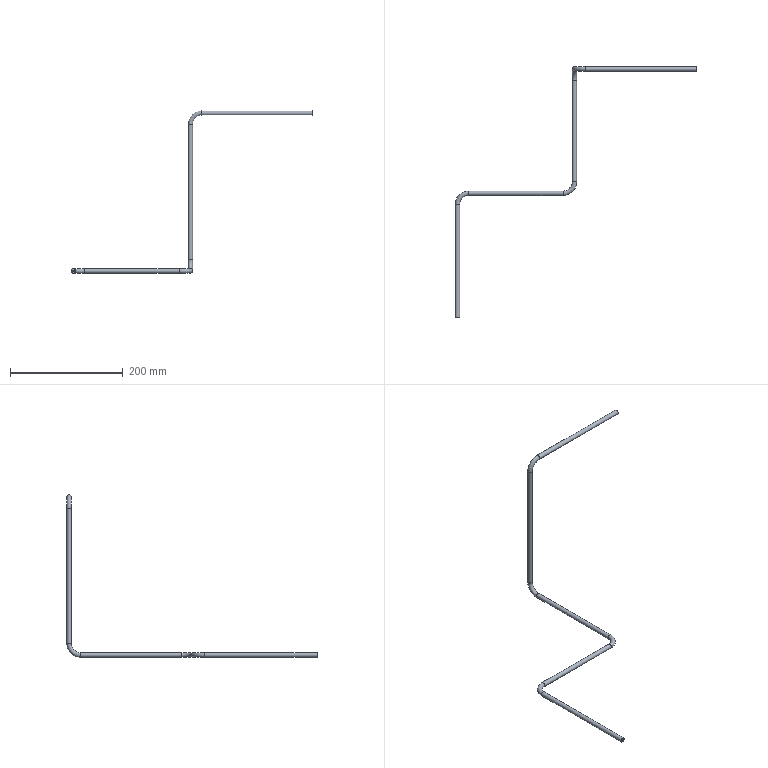Part | NX | features solid 2 | 1 solid | 20 faces | box 428.756 x 443.999 x 288.004 mm | volume 47967 mm3 | cylinder 10 | torus 8 | plane 2 | commonest cylinder face diameters 3 x5 8 x5
STEP:
#1=CARTESIAN_POINT('',(-960.,-15.,-406.));
#2=VERTEX_POINT('',#1);
#3=CARTESIAN_POINT('',(-960.,-15.,-410.));
#4=DIRECTION('',(0.,-1.,0.));
#5=DIRECTION('',(0.,0.,1.));
#6=AXIS2_PLACEMENT_3D('',#3,#4,#5);
#7=CIRCLE('',#6,4.);
#8=EDGE_CURVE('',#2,#2,#7,.T.);
#9=ORIENTED_EDGE('',*,*,#8,.T.);
#10=EDGE_LOOP('',(#9));
#11=FACE_BOUND('',#10,.T.);
#12=CARTESIAN_POINT('',(-960.,-215.,-406.));
#13=VERTEX_POINT('',#12);
#14=CARTESIAN_POINT('',(-960.,-215.,-410.));
#15=DIRECTION('',(0.,-1.,0.));
#16=DIRECTION('',(0.,0.,1.));
#17=AXIS2_PLACEMENT_3D('',#14,#15,#16);
#18=CIRCLE('',#17,4.);
#19=EDGE_CURVE('',#13,#13,#18,.T.);
#20=ORIENTED_EDGE('',*,*,#19,.F.);
#21=EDGE_LOOP('',(#20));
#22=FACE_BOUND('',#21,.T.);
#23=CARTESIAN_POINT('',(-960.,-15.,-410.));
#24=DIRECTION('',(0.,-1.,0.));
#25=DIRECTION('',(0.,0.,-1.));
#26=AXIS2_PLACEMENT_3D('',#23,#24,#25);
#27=CYLINDRICAL_SURFACE('',#26,4.);
#28=ADVANCED_FACE('',(#11,#22),#27,.T.);
#29=CARTESIAN_POINT('',(-960.,-15.,-408.5));
#30=VERTEX_POINT('',#29);
#31=CARTESIAN_POINT('',(-960.,-15.,-410.));
#32=DIRECTION('',(0.,-1.,0.));
#33=DIRECTION('',(0.,0.,1.));
#34=AXIS2_PLACEMENT_3D('',#31,#32,#33);
#35=CIRCLE('',#34,1.5);
#36=EDGE_CURVE('',#30,#30,#35,.T.);
#37=ORIENTED_EDGE('',*,*,#36,.F.);
#38=EDGE_LOOP('',(#37));
#39=FACE_BOUND('',#38,.T.);
#40=CARTESIAN_POINT('',(-960.,-215.,-408.5));
#41=VERTEX_POINT('',#40);
#42=CARTESIAN_POINT('',(-960.,-215.,-410.));
#43=DIRECTION('',(0.,-1.,0.));
#44=DIRECTION('',(0.,0.,1.));
#45=AXIS2_PLACEMENT_3D('',#42,#43,#44);
#46=CIRCLE('',#45,1.5);
#47=EDGE_CURVE('',#41,#41,#46,.T.);
#48=ORIENTED_EDGE('',*,*,#47,.T.);
#49=EDGE_LOOP('',(#48));
#50=FACE_BOUND('',#49,.T.);
#51=CARTESIAN_POINT('',(-960.,-15.,-410.));
#52=DIRECTION('',(0.,-1.,0.));
#53=DIRECTION('',(0.,0.,-1.));
#54=AXIS2_PLACEMENT_3D('',#51,#52,#53);
#55=CYLINDRICAL_SURFACE('',#54,1.5);
#56=ADVANCED_FACE('',(#39,#50),#55,.F.);
#57=CARTESIAN_POINT('',(-940.,5.,-406.));
#58=VERTEX_POINT('',#57);
#59=CARTESIAN_POINT('',(-940.,5.,-410.));
#60=DIRECTION('',(-1.,0.,0.));
#61=DIRECTION('',(0.,0.,1.));
#62=AXIS2_PLACEMENT_3D('',#59,#60,#61);
#63=CIRCLE('',#62,4.);
#64=EDGE_CURVE('',#58,#58,#63,.T.);
#65=ORIENTED_EDGE('',*,*,#64,.T.);
#66=EDGE_LOOP('',(#65));
#67=FACE_BOUND('',#66,.T.);
#68=ORIENTED_EDGE('',*,*,#8,.F.);
#69=EDGE_LOOP('',(#68));
#70=FACE_BOUND('',#69,.T.);
#71=CARTESIAN_POINT('',(-940.,-15.,-410.));
#72=DIRECTION('',(0.,0.,1.));
#73=DIRECTION('',(1.,0.,0.));
#74=AXIS2_PLACEMENT_3D('',#71,#72,#73);
#75=TOROIDAL_SURFACE('',#74,20.,4.);
#76=ADVANCED_FACE('',(#67,#70),#75,.T.);
#77=CARTESIAN_POINT('',(-940.,5.,-408.5));
#78=VERTEX_POINT('',#77);
#79=CARTESIAN_POINT('',(-940.,5.,-410.));
#80=DIRECTION('',(-1.,0.,0.));
#81=DIRECTION('',(0.,0.,1.));
#82=AXIS2_PLACEMENT_3D('',#79,#80,#81);
#83=CIRCLE('',#82,1.5);
#84=EDGE_CURVE('',#78,#78,#83,.T.);
#85=ORIENTED_EDGE('',*,*,#84,.F.);
#86=EDGE_LOOP('',(#85));
#87=FACE_BOUND('',#86,.T.);
#88=ORIENTED_EDGE('',*,*,#36,.T.);
#89=EDGE_LOOP('',(#88));
#90=FACE_BOUND('',#89,.T.);
#91=CARTESIAN_POINT('',(-940.,-15.,-410.));
#92=DIRECTION('',(0.,0.,1.));
#93=DIRECTION('',(1.,0.,0.));
#94=AXIS2_PLACEMENT_3D('',#91,#92,#93);
#95=TOROIDAL_SURFACE('',#94,20.,1.5);
#96=ADVANCED_FACE('',(#87,#90),#95,.F.);
#97=CARTESIAN_POINT('',(-772.5,5.,-406.));
#98=VERTEX_POINT('',#97);
#99=CARTESIAN_POINT('',(-772.5,5.,-410.));
#100=DIRECTION('',(-1.,0.,0.));
#101=DIRECTION('',(0.,0.,1.));
#102=AXIS2_PLACEMENT_3D('',#99,#100,#101);
#103=CIRCLE('',#102,4.);
#104=EDGE_CURVE('',#98,#98,#103,.T.);
#105=ORIENTED_EDGE('',*,*,#104,.T.);
#106=EDGE_LOOP('',(#105));
#107=FACE_BOUND('',#106,.T.);
#108=ORIENTED_EDGE('',*,*,#64,.F.);
#109=EDGE_LOOP('',(#108));
#110=FACE_BOUND('',#109,.T.);
#111=CARTESIAN_POINT('',(-772.5,5.,-410.));
#112=DIRECTION('',(-1.,0.,0.));
#113=DIRECTION('',(0.,0.,1.));
#114=AXIS2_PLACEMENT_3D('',#111,#112,#113);
#115=CYLINDRICAL_SURFACE('',#114,4.);
#116=ADVANCED_FACE('',(#107,#110),#115,.T.);
#117=CARTESIAN_POINT('',(-772.5,5.,-408.5));
#118=VERTEX_POINT('',#117);
#119=CARTESIAN_POINT('',(-772.5,5.,-410.));
#120=DIRECTION('',(-1.,0.,0.));
#121=DIRECTION('',(0.,0.,1.));
#122=AXIS2_PLACEMENT_3D('',#119,#120,#121);
#123=CIRCLE('',#122,1.5);
#124=EDGE_CURVE('',#118,#118,#123,.T.);
#125=ORIENTED_EDGE('',*,*,#124,.F.);
#126=EDGE_LOOP('',(#125));
#127=FACE_BOUND('',#126,.T.);
#128=ORIENTED_EDGE('',*,*,#84,.T.);
#129=EDGE_LOOP('',(#128));
#130=FACE_BOUND('',#129,.T.);
#131=CARTESIAN_POINT('',(-772.5,5.,-410.));
#132=DIRECTION('',(-1.,0.,0.));
#133=DIRECTION('',(0.,0.,1.));
#134=AXIS2_PLACEMENT_3D('',#131,#132,#133);
#135=CYLINDRICAL_SURFACE('',#134,1.5);
#136=ADVANCED_FACE('',(#127,#130),#135,.F.);
#137=CARTESIAN_POINT('',(-752.5,25.,-406.));
#138=VERTEX_POINT('',#137);
#139=CARTESIAN_POINT('',(-752.5,25.,-410.));
#140=DIRECTION('',(0.,-1.,0.));
#141=DIRECTION('',(0.,0.,1.));
#142=AXIS2_PLACEMENT_3D('',#139,#140,#141);
#143=CIRCLE('',#142,4.);
#144=EDGE_CURVE('',#138,#138,#143,.T.);
#145=ORIENTED_EDGE('',*,*,#144,.T.);
#146=EDGE_LOOP('',(#145));
#147=FACE_BOUND('',#146,.T.);
#148=ORIENTED_EDGE('',*,*,#104,.F.);
#149=EDGE_LOOP('',(#148));
#150=FACE_BOUND('',#149,.T.);
#151=CARTESIAN_POINT('',(-772.5,25.,-410.));
#152=DIRECTION('',(0.,0.,-1.));
#153=DIRECTION('',(-1.,0.,0.));
#154=AXIS2_PLACEMENT_3D('',#151,#152,#153);
#155=TOROIDAL_SURFACE('',#154,20.,4.);
#156=ADVANCED_FACE('',(#147,#150),#155,.T.);
#157=CARTESIAN_POINT('',(-752.5,25.,-408.5));
#158=VERTEX_POINT('',#157);
#159=CARTESIAN_POINT('',(-752.5,25.,-410.));
#160=DIRECTION('',(0.,-1.,0.));
#161=DIRECTION('',(0.,0.,1.));
#162=AXIS2_PLACEMENT_3D('',#159,#160,#161);
#163=CIRCLE('',#162,1.5);
#164=EDGE_CURVE('',#158,#158,#163,.T.);
#165=ORIENTED_EDGE('',*,*,#164,.F.);
#166=EDGE_LOOP('',(#165));
#167=FACE_BOUND('',#166,.T.);
#168=ORIENTED_EDGE('',*,*,#124,.T.);
#169=EDGE_LOOP('',(#168));
#170=FACE_BOUND('',#169,.T.);
#171=CARTESIAN_POINT('',(-772.5,25.,-410.));
#172=DIRECTION('',(0.,0.,-1.));
#173=DIRECTION('',(-1.,0.,0.));
#174=AXIS2_PLACEMENT_3D('',#171,#172,#173);
#175=TOROIDAL_SURFACE('',#174,20.,1.5);
#176=ADVANCED_FACE('',(#167,#170),#175,.F.);
#177=CARTESIAN_POINT('',(-752.5,204.999,-406.));
#178=VERTEX_POINT('',#177);
#179=CARTESIAN_POINT('',(-752.5,204.999,-410.));
#180=DIRECTION('',(0.,-1.,0.));
#181=DIRECTION('',(0.,0.,1.));
#182=AXIS2_PLACEMENT_3D('',#179,#180,#181);
#183=CIRCLE('',#182,4.);
#184=EDGE_CURVE('',#178,#178,#183,.T.);
#185=ORIENTED_EDGE('',*,*,#184,.T.);
#186=EDGE_LOOP('',(#185));
#187=FACE_BOUND('',#186,.T.);
#188=ORIENTED_EDGE('',*,*,#144,.F.);
#189=EDGE_LOOP('',(#188));
#190=FACE_BOUND('',#189,.T.);
#191=CARTESIAN_POINT('',(-752.5,204.999,-410.));
#192=DIRECTION('',(0.,-1.,0.));
#193=DIRECTION('',(0.,0.,-1.));
#194=AXIS2_PLACEMENT_3D('',#191,#192,#193);
#195=CYLINDRICAL_SURFACE('',#194,4.);
#196=ADVANCED_FACE('',(#187,#190),#195,.T.);
#197=CARTESIAN_POINT('',(-752.5,204.999,-408.5));
#198=VERTEX_POINT('',#197);
#199=CARTESIAN_POINT('',(-752.5,204.999,-410.));
#200=DIRECTION('',(0.,-1.,0.));
#201=DIRECTION('',(0.,0.,1.));
#202=AXIS2_PLACEMENT_3D('',#199,#200,#201);
#203=CIRCLE('',#202,1.5);
#204=EDGE_CURVE('',#198,#198,#203,.T.);
#205=ORIENTED_EDGE('',*,*,#204,.F.);
#206=EDGE_LOOP('',(#205));
#207=FACE_BOUND('',#206,.T.);
#208=ORIENTED_EDGE('',*,*,#164,.T.);
#209=EDGE_LOOP('',(#208));
#210=FACE_BOUND('',#209,.T.);
#211=CARTESIAN_POINT('',(-752.5,204.999,-410.));
#212=DIRECTION('',(0.,-1.,0.));
#213=DIRECTION('',(0.,0.,-1.));
#214=AXIS2_PLACEMENT_3D('',#211,#212,#213);
#215=CYLINDRICAL_SURFACE('',#214,1.5);
#216=ADVANCED_FACE('',(#207,#210),#215,.F.);
#217=CARTESIAN_POINT('',(-752.5,220.999,-390.));
#218=VERTEX_POINT('',#217);
#219=CARTESIAN_POINT('',(-752.5,224.999,-390.));
#220=DIRECTION('',(0.,0.,-1.));
#221=DIRECTION('',(0.,-1.,0.));
#222=AXIS2_PLACEMENT_3D('',#219,#220,#221);
#223=CIRCLE('',#222,4.);
#224=EDGE_CURVE('',#218,#218,#223,.T.);
#225=ORIENTED_EDGE('',*,*,#224,.T.);
#226=EDGE_LOOP('',(#225));
#227=FACE_BOUND('',#226,.T.);
#228=ORIENTED_EDGE('',*,*,#184,.F.);
#229=EDGE_LOOP('',(#228));
#230=FACE_BOUND('',#229,.T.);
#231=CARTESIAN_POINT('',(-752.5,204.999,-390.));
#232=DIRECTION('',(-1.,0.,0.));
#233=DIRECTION('',(0.,0.,1.));
#234=AXIS2_PLACEMENT_3D('',#231,#232,#233);
#235=TOROIDAL_SURFACE('',#234,20.,4.);
#236=ADVANCED_FACE('',(#227,#230),#235,.T.);
#237=CARTESIAN_POINT('',(-752.5,223.499,-390.));
#238=VERTEX_POINT('',#237);
#239=CARTESIAN_POINT('',(-752.5,224.999,-390.));
#240=DIRECTION('',(0.,0.,-1.));
#241=DIRECTION('',(0.,-1.,0.));
#242=AXIS2_PLACEMENT_3D('',#239,#240,#241);
#243=CIRCLE('',#242,1.5);
#244=EDGE_CURVE('',#238,#238,#243,.T.);
#245=ORIENTED_EDGE('',*,*,#244,.F.);
#246=EDGE_LOOP('',(#245));
#247=FACE_BOUND('',#246,.T.);
#248=ORIENTED_EDGE('',*,*,#204,.T.);
#249=EDGE_LOOP('',(#248));
#250=FACE_BOUND('',#249,.T.);
#251=CARTESIAN_POINT('',(-752.5,204.999,-390.));
#252=DIRECTION('',(-1.,0.,0.));
#253=DIRECTION('',(0.,0.,1.));
#254=AXIS2_PLACEMENT_3D('',#251,#252,#253);
#255=TOROIDAL_SURFACE('',#254,20.,1.5);
#256=ADVANCED_FACE('',(#247,#250),#255,.F.);
#257=CARTESIAN_POINT('',(-752.5,220.999,-149.996));
#258=VERTEX_POINT('',#257);
#259=CARTESIAN_POINT('',(-752.5,224.999,-149.996));
#260=DIRECTION('',(0.,0.,-1.));
#261=DIRECTION('',(0.,-1.,0.));
#262=AXIS2_PLACEMENT_3D('',#259,#260,#261);
#263=CIRCLE('',#262,4.);
#264=EDGE_CURVE('',#258,#258,#263,.T.);
#265=ORIENTED_EDGE('',*,*,#264,.T.);
#266=EDGE_LOOP('',(#265));
#267=FACE_BOUND('',#266,.T.);
#268=ORIENTED_EDGE('',*,*,#224,.F.);
#269=EDGE_LOOP('',(#268));
#270=FACE_BOUND('',#269,.T.);
#271=CARTESIAN_POINT('',(-752.5,224.999,-149.996));
#272=DIRECTION('',(0.,0.,-1.));
#273=DIRECTION('',(-1.,0.,0.));
#274=AXIS2_PLACEMENT_3D('',#271,#272,#273);
#275=CYLINDRICAL_SURFACE('',#274,4.);
#276=ADVANCED_FACE('',(#267,#270),#275,.T.);
#277=CARTESIAN_POINT('',(-752.5,223.499,-149.996));
#278=VERTEX_POINT('',#277);
#279=CARTESIAN_POINT('',(-752.5,224.999,-149.996));
#280=DIRECTION('',(0.,0.,-1.));
#281=DIRECTION('',(0.,-1.,0.));
#282=AXIS2_PLACEMENT_3D('',#279,#280,#281);
#283=CIRCLE('',#282,1.5);
#284=EDGE_CURVE('',#278,#278,#283,.T.);
#285=ORIENTED_EDGE('',*,*,#284,.F.);
#286=EDGE_LOOP('',(#285));
#287=FACE_BOUND('',#286,.T.);
#288=ORIENTED_EDGE('',*,*,#244,.T.);
#289=EDGE_LOOP('',(#288));
#290=FACE_BOUND('',#289,.T.);
#291=CARTESIAN_POINT('',(-752.5,224.999,-149.996));
#292=DIRECTION('',(0.,0.,-1.));
#293=DIRECTION('',(-1.,0.,0.));
#294=AXIS2_PLACEMENT_3D('',#291,#292,#293);
#295=CYLINDRICAL_SURFACE('',#294,1.5);
#296=ADVANCED_FACE('',(#287,#290),#295,.F.);
#297=CARTESIAN_POINT('',(-732.5,220.999,-129.996));
#298=VERTEX_POINT('',#297);
#299=CARTESIAN_POINT('',(-732.5,224.999,-129.996));
#300=DIRECTION('',(-1.,0.,0.));
#301=DIRECTION('',(0.,-1.,0.));
#302=AXIS2_PLACEMENT_3D('',#299,#300,#301);
#303=CIRCLE('',#302,4.);
#304=EDGE_CURVE('',#298,#298,#303,.T.);
#305=ORIENTED_EDGE('',*,*,#304,.T.);
#306=EDGE_LOOP('',(#305));
#307=FACE_BOUND('',#306,.T.);
#308=ORIENTED_EDGE('',*,*,#264,.F.);
#309=EDGE_LOOP('',(#308));
#310=FACE_BOUND('',#309,.T.);
#311=CARTESIAN_POINT('',(-732.5,224.999,-149.996));
#312=DIRECTION('',(0.,-1.,0.));
#313=DIRECTION('',(0.,0.,-1.));
#314=AXIS2_PLACEMENT_3D('',#311,#312,#313);
#315=TOROIDAL_SURFACE('',#314,20.,4.);
#316=ADVANCED_FACE('',(#307,#310),#315,.T.);
#317=CARTESIAN_POINT('',(-732.5,223.499,-129.996));
#318=VERTEX_POINT('',#317);
#319=CARTESIAN_POINT('',(-732.5,224.999,-129.996));
#320=DIRECTION('',(-1.,0.,0.));
#321=DIRECTION('',(0.,-1.,0.));
#322=AXIS2_PLACEMENT_3D('',#319,#320,#321);
#323=CIRCLE('',#322,1.5);
#324=EDGE_CURVE('',#318,#318,#323,.T.);
#325=ORIENTED_EDGE('',*,*,#324,.F.);
#326=EDGE_LOOP('',(#325));
#327=FACE_BOUND('',#326,.T.);
#328=ORIENTED_EDGE('',*,*,#284,.T.);
#329=EDGE_LOOP('',(#328));
#330=FACE_BOUND('',#329,.T.);
#331=CARTESIAN_POINT('',(-732.5,224.999,-149.996));
#332=DIRECTION('',(0.,-1.,0.));
#333=DIRECTION('',(0.,0.,-1.));
#334=AXIS2_PLACEMENT_3D('',#331,#332,#333);
#335=TOROIDAL_SURFACE('',#334,20.,1.5);
#336=ADVANCED_FACE('',(#327,#330),#335,.F.);
#337=ORIENTED_EDGE('',*,*,#324,.T.);
#338=EDGE_LOOP('',(#337));
#339=FACE_BOUND('',#338,.T.);
#340=CARTESIAN_POINT('',(-535.244,223.499,-129.996));
#341=VERTEX_POINT('',#340);
#342=CARTESIAN_POINT('',(-535.244,224.999,-129.996));
#343=DIRECTION('',(-1.,0.,0.));
#344=DIRECTION('',(0.,-1.,0.));
#345=AXIS2_PLACEMENT_3D('',#342,#343,#344);
#346=CIRCLE('',#345,1.5);
#347=EDGE_CURVE('',#341,#341,#346,.T.);
#348=ORIENTED_EDGE('',*,*,#347,.F.);
#349=EDGE_LOOP('',(#348));
#350=FACE_BOUND('',#349,.T.);
#351=CARTESIAN_POINT('',(-732.5,224.999,-129.996));
#352=DIRECTION('',(1.,0.,0.));
#353=DIRECTION('',(0.,1.,0.));
#354=AXIS2_PLACEMENT_3D('',#351,#352,#353);
#355=CYLINDRICAL_SURFACE('',#354,1.5);
#356=ADVANCED_FACE('',(#339,#350),#355,.F.);
#357=ORIENTED_EDGE('',*,*,#304,.F.);
#358=EDGE_LOOP('',(#357));
#359=FACE_BOUND('',#358,.T.);
#360=CARTESIAN_POINT('',(-535.244,220.999,-129.996));
#361=VERTEX_POINT('',#360);
#362=CARTESIAN_POINT('',(-535.244,224.999,-129.996));
#363=DIRECTION('',(-1.,0.,0.));
#364=DIRECTION('',(0.,-1.,0.));
#365=AXIS2_PLACEMENT_3D('',#362,#363,#364);
#366=CIRCLE('',#365,4.);
#367=EDGE_CURVE('',#361,#361,#366,.T.);
#368=ORIENTED_EDGE('',*,*,#367,.T.);
#369=EDGE_LOOP('',(#368));
#370=FACE_BOUND('',#369,.T.);
#371=CARTESIAN_POINT('',(-732.5,224.999,-129.996));
#372=DIRECTION('',(1.,0.,0.));
#373=DIRECTION('',(0.,1.,0.));
#374=AXIS2_PLACEMENT_3D('',#371,#372,#373);
#375=CYLINDRICAL_SURFACE('',#374,4.);
#376=ADVANCED_FACE('',(#359,#370),#375,.T.);
#377=ORIENTED_EDGE('',*,*,#47,.F.);
#378=EDGE_LOOP('',(#377));
#379=FACE_BOUND('',#378,.T.);
#380=ORIENTED_EDGE('',*,*,#19,.T.);
#381=EDGE_LOOP('',(#380));
#382=FACE_BOUND('',#381,.T.);
#383=CARTESIAN_POINT('',(-960.,-215.,-410.));
#384=DIRECTION('',(0.,-1.,0.));
#385=DIRECTION('',(0.,0.,1.));
#386=AXIS2_PLACEMENT_3D('',#383,#384,#385);
#387=PLANE('',#386);
#388=ADVANCED_FACE('',(#379,#382),#387,.T.);
#389=ORIENTED_EDGE('',*,*,#347,.T.);
#390=EDGE_LOOP('',(#389));
#391=FACE_BOUND('',#390,.T.);
#392=ORIENTED_EDGE('',*,*,#367,.F.);
#393=EDGE_LOOP('',(#392));
#394=FACE_BOUND('',#393,.T.);
#395=CARTESIAN_POINT('',(-535.244,224.999,-129.996));
#396=DIRECTION('',(-1.,0.,0.));
#397=DIRECTION('',(0.,-1.,0.));
#398=AXIS2_PLACEMENT_3D('',#395,#396,#397);
#399=PLANE('',#398);
#400=ADVANCED_FACE('',(#391,#394),#399,.F.);
#401=CLOSED_SHELL('',(#28,#56,#76,#96,#116,#136,#156,#176,#196,#216,#236,#256,#276,#296,#316,#336,#356,#376,#388,#400));
#402=MANIFOLD_SOLID_BREP('',#401);
#403=(LENGTH_UNIT()NAMED_UNIT(*)SI_UNIT(.MILLI.,.METRE.));
#404=UNCERTAINTY_MEASURE_WITH_UNIT(LENGTH_MEASURE(0.00001),#403,'','');
#405=(NAMED_UNIT(*)PLANE_ANGLE_UNIT()SI_UNIT($,.RADIAN.));
#406=(NAMED_UNIT(*)SI_UNIT($,.STERADIAN.)SOLID_ANGLE_UNIT());
#407=(GEOMETRIC_REPRESENTATION_CONTEXT(3)GLOBAL_UNCERTAINTY_ASSIGNED_CONTEXT((#404))GLOBAL_UNIT_ASSIGNED_CONTEXT((#403,#405,#406))REPRESENTATION_CONTEXT('',''));
#408=ADVANCED_BREP_SHAPE_REPRESENTATION('',(#402),#407);